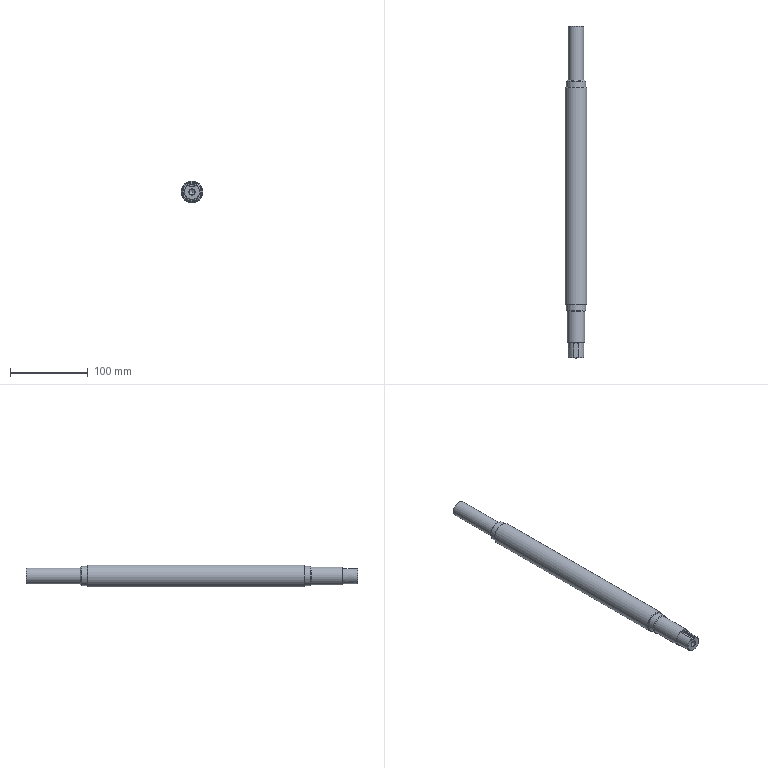Part | NX | features DATUM_CSYS 3, CHAMFER 2, EXTRUDE 2, SKETCH 2, FACE_BLEND 1, HOLE PACKAGE 1, SIMPLE HOLE 1, SWP104 1, SYMBOLIC_THREAD 1 | 1 solid | 25 faces | box 28 x 428 x 28 mm | volume 224992 mm3 | plane 9 | cylinder 8 | cone 8 | commonest cylinder face diameters 20 x2 25 x2 6 x1 7.2 x1 23 x1 28 x1
STEP:
#1=CARTESIAN_POINT('',(0.,428.,9.5));
#2=VERTEX_POINT('',#1);
#3=CARTESIAN_POINT('',(0.,428.,0.));
#4=DIRECTION('',(0.,1.,0.));
#5=DIRECTION('',(0.,0.,1.));
#6=AXIS2_PLACEMENT_3D('',#3,#4,#5);
#7=CIRCLE('',#6,9.5);
#8=EDGE_CURVE('',#2,#2,#7,.T.);
#9=ORIENTED_EDGE('',*,*,#8,.T.);
#10=EDGE_LOOP('',(#9));
#11=FACE_BOUND('',#10,.T.);
#12=CARTESIAN_POINT('',(0.,428.,0.));
#13=DIRECTION('',(0.,1.,0.));
#14=DIRECTION('',(0.,0.,1.));
#15=AXIS2_PLACEMENT_3D('',#12,#13,#14);
#16=PLANE('',#15);
#17=ADVANCED_FACE('',(#11),#16,.T.);
#18=CARTESIAN_POINT('',(0.,427.5,10.));
#19=VERTEX_POINT('',#18);
#20=CARTESIAN_POINT('',(0.,427.5,0.));
#21=DIRECTION('',(0.,1.,0.));
#22=DIRECTION('',(0.,0.,1.));
#23=AXIS2_PLACEMENT_3D('',#20,#21,#22);
#24=CIRCLE('',#23,10.);
#25=EDGE_CURVE('',#19,#19,#24,.F.);
#26=ORIENTED_EDGE('',*,*,#25,.T.);
#27=EDGE_LOOP('',(#26));
#28=FACE_BOUND('',#27,.T.);
#29=CARTESIAN_POINT('',(0.,358.,10.));
#30=VERTEX_POINT('',#29);
#31=CARTESIAN_POINT('',(0.,358.,0.));
#32=DIRECTION('',(0.,1.,0.));
#33=DIRECTION('',(0.,0.,1.));
#34=AXIS2_PLACEMENT_3D('',#31,#32,#33);
#35=CIRCLE('',#34,10.);
#36=EDGE_CURVE('',#30,#30,#35,.T.);
#37=ORIENTED_EDGE('',*,*,#36,.T.);
#38=EDGE_LOOP('',(#37));
#39=FACE_BOUND('',#38,.T.);
#40=CARTESIAN_POINT('',(0.,0.,0.));
#41=DIRECTION('',(0.,1.,0.));
#42=DIRECTION('',(0.,0.,1.));
#43=AXIS2_PLACEMENT_3D('',#40,#41,#42);
#44=CYLINDRICAL_SURFACE('',#43,10.);
#45=ADVANCED_FACE('',(#28,#39),#44,.T.);
#46=CARTESIAN_POINT('',(0.,358.,-11.5));
#47=VERTEX_POINT('',#46);
#48=CARTESIAN_POINT('',(0.,358.,0.));
#49=DIRECTION('',(0.,-1.,0.));
#50=DIRECTION('',(0.,0.,-1.));
#51=AXIS2_PLACEMENT_3D('',#48,#49,#50);
#52=CIRCLE('',#51,11.5);
#53=EDGE_CURVE('',#47,#47,#52,.F.);
#54=ORIENTED_EDGE('',*,*,#53,.T.);
#55=EDGE_LOOP('',(#54));
#56=FACE_BOUND('',#55,.T.);
#57=ORIENTED_EDGE('',*,*,#36,.F.);
#58=EDGE_LOOP('',(#57));
#59=FACE_BOUND('',#58,.T.);
#60=CARTESIAN_POINT('',(-12.5,358.,0.));
#61=DIRECTION('',(0.,-1.,0.));
#62=DIRECTION('',(0.,0.,-1.));
#63=AXIS2_PLACEMENT_3D('',#60,#61,#62);
#64=PLANE('',#63);
#65=ADVANCED_FACE('',(#56,#59),#64,.F.);
#66=CARTESIAN_POINT('',(0.,357.,-12.5));
#67=VERTEX_POINT('',#66);
#68=CARTESIAN_POINT('',(0.,357.,0.));
#69=DIRECTION('',(0.,-1.,0.));
#70=DIRECTION('',(0.,0.,-1.));
#71=AXIS2_PLACEMENT_3D('',#68,#69,#70);
#72=CIRCLE('',#71,12.5);
#73=EDGE_CURVE('',#67,#67,#72,.T.);
#74=ORIENTED_EDGE('',*,*,#73,.T.);
#75=EDGE_LOOP('',(#74));
#76=FACE_BOUND('',#75,.T.);
#77=CARTESIAN_POINT('',(0.,349.,12.5));
#78=VERTEX_POINT('',#77);
#79=CARTESIAN_POINT('',(0.,349.,0.));
#80=DIRECTION('',(0.,1.,0.));
#81=DIRECTION('',(0.,0.,1.));
#82=AXIS2_PLACEMENT_3D('',#79,#80,#81);
#83=CIRCLE('',#82,12.5);
#84=EDGE_CURVE('',#78,#78,#83,.T.);
#85=ORIENTED_EDGE('',*,*,#84,.T.);
#86=EDGE_LOOP('',(#85));
#87=FACE_BOUND('',#86,.T.);
#88=CARTESIAN_POINT('',(0.,0.,0.));
#89=DIRECTION('',(0.,1.,0.));
#90=DIRECTION('',(0.,0.,1.));
#91=AXIS2_PLACEMENT_3D('',#88,#89,#90);
#92=CYLINDRICAL_SURFACE('',#91,12.5);
#93=ADVANCED_FACE('',(#76,#87),#92,.T.);
#94=CARTESIAN_POINT('',(0.,349.,-13.5));
#95=VERTEX_POINT('',#94);
#96=CARTESIAN_POINT('',(0.,349.,0.));
#97=DIRECTION('',(0.,-1.,0.));
#98=DIRECTION('',(0.,0.,-1.));
#99=AXIS2_PLACEMENT_3D('',#96,#97,#98);
#100=CIRCLE('',#99,13.5);
#101=EDGE_CURVE('',#95,#95,#100,.F.);
#102=ORIENTED_EDGE('',*,*,#101,.T.);
#103=EDGE_LOOP('',(#102));
#104=FACE_BOUND('',#103,.T.);
#105=ORIENTED_EDGE('',*,*,#84,.F.);
#106=EDGE_LOOP('',(#105));
#107=FACE_BOUND('',#106,.T.);
#108=CARTESIAN_POINT('',(-14.,349.,0.));
#109=DIRECTION('',(0.,-1.,0.));
#110=DIRECTION('',(0.,0.,-1.));
#111=AXIS2_PLACEMENT_3D('',#108,#109,#110);
#112=PLANE('',#111);
#113=ADVANCED_FACE('',(#104,#107),#112,.F.);
#114=CARTESIAN_POINT('',(0.,348.5,-14.));
#115=VERTEX_POINT('',#114);
#116=CARTESIAN_POINT('',(0.,348.5,0.));
#117=DIRECTION('',(0.,-1.,0.));
#118=DIRECTION('',(0.,0.,-1.));
#119=AXIS2_PLACEMENT_3D('',#116,#117,#118);
#120=CIRCLE('',#119,14.);
#121=EDGE_CURVE('',#115,#115,#120,.T.);
#122=ORIENTED_EDGE('',*,*,#121,.T.);
#123=EDGE_LOOP('',(#122));
#124=FACE_BOUND('',#123,.T.);
#125=CARTESIAN_POINT('',(0.,69.5,14.));
#126=VERTEX_POINT('',#125);
#127=CARTESIAN_POINT('',(0.,69.5,0.));
#128=DIRECTION('',(0.,1.,0.));
#129=DIRECTION('',(0.,0.,1.));
#130=AXIS2_PLACEMENT_3D('',#127,#128,#129);
#131=CIRCLE('',#130,14.);
#132=EDGE_CURVE('',#126,#126,#131,.T.);
#133=ORIENTED_EDGE('',*,*,#132,.T.);
#134=EDGE_LOOP('',(#133));
#135=FACE_BOUND('',#134,.T.);
#136=CARTESIAN_POINT('',(0.,0.,0.));
#137=DIRECTION('',(0.,1.,0.));
#138=DIRECTION('',(0.,0.,1.));
#139=AXIS2_PLACEMENT_3D('',#136,#137,#138);
#140=CYLINDRICAL_SURFACE('',#139,14.);
#141=ADVANCED_FACE('',(#124,#135),#140,.T.);
#142=CARTESIAN_POINT('',(0.,69.,13.5));
#143=VERTEX_POINT('',#142);
#144=CARTESIAN_POINT('',(0.,69.,0.));
#145=DIRECTION('',(0.,1.,0.));
#146=DIRECTION('',(0.,0.,1.));
#147=AXIS2_PLACEMENT_3D('',#144,#145,#146);
#148=CIRCLE('',#147,13.5);
#149=EDGE_CURVE('',#143,#143,#148,.F.);
#150=ORIENTED_EDGE('',*,*,#149,.T.);
#151=EDGE_LOOP('',(#150));
#152=FACE_BOUND('',#151,.T.);
#153=CARTESIAN_POINT('',(0.,69.,12.5));
#154=VERTEX_POINT('',#153);
#155=CARTESIAN_POINT('',(0.,69.,0.));
#156=DIRECTION('',(0.,1.,0.));
#157=DIRECTION('',(0.,0.,1.));
#158=AXIS2_PLACEMENT_3D('',#155,#156,#157);
#159=CIRCLE('',#158,12.5);
#160=EDGE_CURVE('',#154,#154,#159,.T.);
#161=ORIENTED_EDGE('',*,*,#160,.T.);
#162=EDGE_LOOP('',(#161));
#163=FACE_BOUND('',#162,.T.);
#164=CARTESIAN_POINT('',(-12.5,69.,0.));
#165=DIRECTION('',(0.,1.,0.));
#166=DIRECTION('',(0.,0.,1.));
#167=AXIS2_PLACEMENT_3D('',#164,#165,#166);
#168=PLANE('',#167);
#169=ADVANCED_FACE('',(#152,#163),#168,.F.);
#170=CARTESIAN_POINT('',(0.,61.,12.5));
#171=VERTEX_POINT('',#170);
#172=CARTESIAN_POINT('',(0.,61.,0.));
#173=DIRECTION('',(0.,1.,0.));
#174=DIRECTION('',(0.,0.,1.));
#175=AXIS2_PLACEMENT_3D('',#172,#173,#174);
#176=CIRCLE('',#175,12.5);
#177=EDGE_CURVE('',#171,#171,#176,.T.);
#178=ORIENTED_EDGE('',*,*,#177,.T.);
#179=EDGE_LOOP('',(#178));
#180=FACE_BOUND('',#179,.T.);
#181=ORIENTED_EDGE('',*,*,#160,.F.);
#182=EDGE_LOOP('',(#181));
#183=FACE_BOUND('',#182,.T.);
#184=CARTESIAN_POINT('',(0.,0.,0.));
#185=DIRECTION('',(0.,1.,0.));
#186=DIRECTION('',(0.,0.,1.));
#187=AXIS2_PLACEMENT_3D('',#184,#185,#186);
#188=CYLINDRICAL_SURFACE('',#187,12.5);
#189=ADVANCED_FACE('',(#180,#183),#188,.T.);
#190=ORIENTED_EDGE('',*,*,#25,.F.);
#191=EDGE_LOOP('',(#190));
#192=FACE_BOUND('',#191,.T.);
#193=ORIENTED_EDGE('',*,*,#8,.F.);
#194=EDGE_LOOP('',(#193));
#195=FACE_BOUND('',#194,.T.);
#196=CARTESIAN_POINT('',(0.,428.,0.));
#197=DIRECTION('',(0.,-1.,0.));
#198=DIRECTION('',(0.,0.,-1.));
#199=AXIS2_PLACEMENT_3D('',#196,#197,#198);
#200=CONICAL_SURFACE('',#199,9.5,0.7854);
#201=ADVANCED_FACE('',(#192,#195),#200,.T.);
#202=ORIENTED_EDGE('',*,*,#121,.F.);
#203=EDGE_LOOP('',(#202));
#204=FACE_BOUND('',#203,.T.);
#205=ORIENTED_EDGE('',*,*,#101,.F.);
#206=EDGE_LOOP('',(#205));
#207=FACE_BOUND('',#206,.T.);
#208=CARTESIAN_POINT('',(0.,349.,0.));
#209=DIRECTION('',(0.,-1.,0.));
#210=DIRECTION('',(0.,0.,-1.));
#211=AXIS2_PLACEMENT_3D('',#208,#209,#210);
#212=CONICAL_SURFACE('',#211,13.5,0.7854);
#213=ADVANCED_FACE('',(#204,#207),#212,.T.);
#214=ORIENTED_EDGE('',*,*,#149,.F.);
#215=EDGE_LOOP('',(#214));
#216=FACE_BOUND('',#215,.T.);
#217=ORIENTED_EDGE('',*,*,#132,.F.);
#218=EDGE_LOOP('',(#217));
#219=FACE_BOUND('',#218,.T.);
#220=CARTESIAN_POINT('',(0.,69.5,0.));
#221=DIRECTION('',(0.,1.,0.));
#222=DIRECTION('',(0.,0.,1.));
#223=AXIS2_PLACEMENT_3D('',#220,#221,#222);
#224=CONICAL_SURFACE('',#223,14.,0.7854);
#225=ADVANCED_FACE('',(#216,#219),#224,.T.);
#226=CARTESIAN_POINT('',(0.,60.,11.5));
#227=VERTEX_POINT('',#226);
#228=CARTESIAN_POINT('',(0.,60.,0.));
#229=DIRECTION('',(0.,1.,0.));
#230=DIRECTION('',(0.,0.,1.));
#231=AXIS2_PLACEMENT_3D('',#228,#229,#230);
#232=CIRCLE('',#231,11.5);
#233=EDGE_CURVE('',#227,#227,#232,.F.);
#234=ORIENTED_EDGE('',*,*,#233,.F.);
#235=EDGE_LOOP('',(#234));
#236=FACE_BOUND('',#235,.T.);
#237=ORIENTED_EDGE('',*,*,#177,.F.);
#238=EDGE_LOOP('',(#237));
#239=FACE_BOUND('',#238,.T.);
#240=CARTESIAN_POINT('',(0.,61.,0.));
#241=DIRECTION('',(0.,1.,0.));
#242=DIRECTION('',(0.,0.,1.));
#243=AXIS2_PLACEMENT_3D('',#240,#241,#242);
#244=CONICAL_SURFACE('',#243,12.5,0.7854);
#245=ADVANCED_FACE('',(#236,#239),#244,.T.);
#246=ORIENTED_EDGE('',*,*,#73,.F.);
#247=EDGE_LOOP('',(#246));
#248=FACE_BOUND('',#247,.T.);
#249=ORIENTED_EDGE('',*,*,#53,.F.);
#250=EDGE_LOOP('',(#249));
#251=FACE_BOUND('',#250,.T.);
#252=CARTESIAN_POINT('',(0.,358.,0.));
#253=DIRECTION('',(0.,-1.,0.));
#254=DIRECTION('',(0.,0.,-1.));
#255=AXIS2_PLACEMENT_3D('',#252,#253,#254);
#256=CONICAL_SURFACE('',#255,11.5,0.7854);
#257=ADVANCED_FACE('',(#248,#251),#256,.T.);
#258=CARTESIAN_POINT('',(0.,20.,-11.5));
#259=VERTEX_POINT('',#258);
#260=CARTESIAN_POINT('',(0.,20.,0.));
#261=DIRECTION('',(0.,-1.,0.));
#262=DIRECTION('',(0.,0.,-1.));
#263=AXIS2_PLACEMENT_3D('',#260,#261,#262);
#264=CIRCLE('',#263,11.5);
#265=EDGE_CURVE('',#259,#259,#264,.T.);
#266=ORIENTED_EDGE('',*,*,#265,.T.);
#267=EDGE_LOOP('',(#266));
#268=FACE_BOUND('',#267,.T.);
#269=CARTESIAN_POINT('',(0.,20.,10.));
#270=VERTEX_POINT('',#269);
#271=CARTESIAN_POINT('',(0.,20.,0.));
#272=DIRECTION('',(0.,-1.,0.));
#273=DIRECTION('',(0.,0.,-1.));
#274=AXIS2_PLACEMENT_3D('',#271,#272,#273);
#275=CIRCLE('',#274,10.);
#276=EDGE_CURVE('',#270,#270,#275,.T.);
#277=ORIENTED_EDGE('',*,*,#276,.F.);
#278=EDGE_LOOP('',(#277));
#279=FACE_BOUND('',#278,.T.);
#280=CARTESIAN_POINT('',(0.,20.,0.));
#281=DIRECTION('',(0.,-1.,0.));
#282=DIRECTION('',(0.,0.,-1.));
#283=AXIS2_PLACEMENT_3D('',#280,#281,#282);
#284=PLANE('',#283);
#285=ADVANCED_FACE('',(#268,#279),#284,.T.);
#286=ORIENTED_EDGE('',*,*,#265,.F.);
#287=EDGE_LOOP('',(#286));
#288=FACE_BOUND('',#287,.T.);
#289=ORIENTED_EDGE('',*,*,#233,.T.);
#290=EDGE_LOOP('',(#289));
#291=FACE_BOUND('',#290,.T.);
#292=CARTESIAN_POINT('',(0.,20.,0.));
#293=DIRECTION('',(0.,1.,0.));
#294=DIRECTION('',(0.,0.,1.));
#295=AXIS2_PLACEMENT_3D('',#292,#293,#294);
#296=CYLINDRICAL_SURFACE('',#295,11.5);
#297=ADVANCED_FACE('',(#288,#291),#296,.T.);
#298=CARTESIAN_POINT('',(0.,15.,3.6));
#299=VERTEX_POINT('',#298);
#300=CARTESIAN_POINT('',(0.,15.,0.));
#301=DIRECTION('',(0.,1.,0.));
#302=DIRECTION('',(0.,0.,1.));
#303=AXIS2_PLACEMENT_3D('',#300,#301,#302);
#304=CIRCLE('',#303,3.6);
#305=EDGE_CURVE('',#299,#299,#304,.F.);
#306=ORIENTED_EDGE('',*,*,#305,.T.);
#307=EDGE_LOOP('',(#306));
#308=FACE_BOUND('',#307,.T.);
#309=CARTESIAN_POINT('',(0.,17.163,0.));
#310=VERTEX_POINT('',#309);
#311=VERTEX_LOOP('',#310);
#312=FACE_BOUND('',#311,.T.);
#313=CARTESIAN_POINT('',(0.,15.,0.));
#314=DIRECTION('',(0.,-1.,0.));
#315=DIRECTION('',(0.,0.,-1.));
#316=AXIS2_PLACEMENT_3D('',#313,#314,#315);
#317=CONICAL_SURFACE('',#316,3.6,1.03);
#318=ADVANCED_FACE('',(#308,#312),#317,.F.);
#319=CARTESIAN_POINT('',(0.,0.4,3.6));
#320=VERTEX_POINT('',#319);
#321=CARTESIAN_POINT('',(0.,0.4,0.));
#322=DIRECTION('',(0.,1.,0.));
#323=DIRECTION('',(0.,0.,1.));
#324=AXIS2_PLACEMENT_3D('',#321,#322,#323);
#325=CIRCLE('',#324,3.6);
#326=EDGE_CURVE('',#320,#320,#325,.F.);
#327=ORIENTED_EDGE('',*,*,#326,.T.);
#328=EDGE_LOOP('',(#327));
#329=FACE_BOUND('',#328,.T.);
#330=ORIENTED_EDGE('',*,*,#305,.F.);
#331=EDGE_LOOP('',(#330));
#332=FACE_BOUND('',#331,.T.);
#333=CARTESIAN_POINT('',(0.,0.,0.));
#334=DIRECTION('',(0.,1.,0.));
#335=DIRECTION('',(0.,0.,1.));
#336=AXIS2_PLACEMENT_3D('',#333,#334,#335);
#337=CYLINDRICAL_SURFACE('',#336,3.6);
#338=ADVANCED_FACE('',(#329,#332),#337,.F.);
#339=ORIENTED_EDGE('',*,*,#326,.F.);
#340=EDGE_LOOP('',(#339));
#341=FACE_BOUND('',#340,.T.);
#342=CARTESIAN_POINT('',(0.,0.,4.));
#343=VERTEX_POINT('',#342);
#344=CARTESIAN_POINT('',(0.,0.,0.));
#345=DIRECTION('',(0.,1.,0.));
#346=DIRECTION('',(0.,0.,1.));
#347=AXIS2_PLACEMENT_3D('',#344,#345,#346);
#348=CIRCLE('',#347,4.);
#349=EDGE_CURVE('',#343,#343,#348,.T.);
#350=ORIENTED_EDGE('',*,*,#349,.F.);
#351=EDGE_LOOP('',(#350));
#352=FACE_BOUND('',#351,.T.);
#353=CARTESIAN_POINT('',(0.,0.,0.));
#354=DIRECTION('',(0.,-1.,0.));
#355=DIRECTION('',(0.,0.,-1.));
#356=AXIS2_PLACEMENT_3D('',#353,#354,#355);
#357=CONICAL_SURFACE('',#356,4.,0.7854);
#358=ADVANCED_FACE('',(#341,#352),#357,.F.);
#359=ORIENTED_EDGE('',*,*,#349,.T.);
#360=EDGE_LOOP('',(#359));
#361=FACE_BOUND('',#360,.T.);
#362=CARTESIAN_POINT('',(-3.,0.,9.014));
#363=VERTEX_POINT('',#362);
#364=CARTESIAN_POINT('',(-3.,0.,6.5));
#365=VERTEX_POINT('',#364);
#366=CARTESIAN_POINT('',(-3.,0.,21.5));
#367=DIRECTION('',(0.,0.,-1.));
#368=VECTOR('',#367,1000.);
#369=LINE('',#366,#368);
#370=EDGE_CURVE('',#363,#365,#369,.T.);
#371=ORIENTED_EDGE('',*,*,#370,.F.);
#372=CARTESIAN_POINT('',(3.,0.,9.014));
#373=VERTEX_POINT('',#372);
#374=CARTESIAN_POINT('',(0.,0.,0.));
#375=DIRECTION('',(0.,1.,0.));
#376=DIRECTION('',(0.,0.,1.));
#377=AXIS2_PLACEMENT_3D('',#374,#375,#376);
#378=CIRCLE('',#377,9.5);
#379=EDGE_CURVE('',#363,#373,#378,.F.);
#380=ORIENTED_EDGE('',*,*,#379,.T.);
#381=CARTESIAN_POINT('',(3.,0.,6.5));
#382=VERTEX_POINT('',#381);
#383=CARTESIAN_POINT('',(3.,0.,6.5));
#384=DIRECTION('',(0.,0.,1.));
#385=VECTOR('',#384,1000.);
#386=LINE('',#383,#385);
#387=EDGE_CURVE('',#382,#373,#386,.T.);
#388=ORIENTED_EDGE('',*,*,#387,.F.);
#389=CARTESIAN_POINT('',(-3.,0.,6.5));
#390=DIRECTION('',(1.,0.,0.));
#391=VECTOR('',#390,1000.);
#392=LINE('',#389,#391);
#393=EDGE_CURVE('',#365,#382,#392,.T.);
#394=ORIENTED_EDGE('',*,*,#393,.F.);
#395=EDGE_LOOP('',(#371,#380,#388,#394));
#396=FACE_BOUND('',#395,.T.);
#397=CARTESIAN_POINT('',(0.,0.,0.));
#398=DIRECTION('',(0.,1.,0.));
#399=DIRECTION('',(0.,0.,1.));
#400=AXIS2_PLACEMENT_3D('',#397,#398,#399);
#401=PLANE('',#400);
#402=ADVANCED_FACE('',(#361,#396),#401,.F.);
#403=CARTESIAN_POINT('',(3.,17.,6.5));
#404=VERTEX_POINT('',#403);
#405=CARTESIAN_POINT('',(3.,20.,6.5));
#406=DIRECTION('',(0.,-1.,0.));
#407=VECTOR('',#406,1000.);
#408=LINE('',#405,#407);
#409=EDGE_CURVE('',#382,#404,#408,.F.);
#410=ORIENTED_EDGE('',*,*,#409,.T.);
#411=CARTESIAN_POINT('',(-3.,17.,6.5));
#412=VERTEX_POINT('',#411);
#413=CARTESIAN_POINT('',(0.,17.,6.5));
#414=DIRECTION('',(0.,0.,-1.));
#415=DIRECTION('',(-1.,0.,0.));
#416=AXIS2_PLACEMENT_3D('',#413,#414,#415);
#417=CIRCLE('',#416,3.);
#418=EDGE_CURVE('',#404,#412,#417,.F.);
#419=ORIENTED_EDGE('',*,*,#418,.T.);
#420=CARTESIAN_POINT('',(-3.,20.,6.5));
#421=DIRECTION('',(0.,-1.,0.));
#422=VECTOR('',#421,1000.);
#423=LINE('',#420,#422);
#424=EDGE_CURVE('',#365,#412,#423,.F.);
#425=ORIENTED_EDGE('',*,*,#424,.F.);
#426=ORIENTED_EDGE('',*,*,#393,.T.);
#427=EDGE_LOOP('',(#410,#419,#425,#426));
#428=FACE_BOUND('',#427,.T.);
#429=CARTESIAN_POINT('',(-3.,20.,6.5));
#430=DIRECTION('',(0.,0.,-1.));
#431=DIRECTION('',(-1.,0.,0.));
#432=AXIS2_PLACEMENT_3D('',#429,#430,#431);
#433=PLANE('',#432);
#434=ADVANCED_FACE('',(#428),#433,.F.);
#435=CARTESIAN_POINT('',(-3.,0.5,9.539));
#436=VERTEX_POINT('',#435);
#437=CARTESIAN_POINT('',(-3.,17.,9.539));
#438=VERTEX_POINT('',#437);
#439=CARTESIAN_POINT('',(-3.,0.,9.539));
#440=DIRECTION('',(0.,1.,0.));
#441=VECTOR('',#440,1000.);
#442=LINE('',#439,#441);
#443=EDGE_CURVE('',#436,#438,#442,.T.);
#444=ORIENTED_EDGE('',*,*,#443,.F.);
#445=CARTESIAN_POINT('',(-3.,0.5,9.539));
#446=CARTESIAN_POINT('',(-3.,0.3331,9.364));
#447=CARTESIAN_POINT('',(-3.,0.1664,9.189));
#448=CARTESIAN_POINT('',(-3.,0.,9.014));
#449=B_SPLINE_CURVE_WITH_KNOTS('',3,(#445,#446,#447,#448),.UNSPECIFIED.,.F.,.F.,(4,4),(0.,0.0007254),.UNSPECIFIED.);
#450=EDGE_CURVE('',#436,#363,#449,.T.);
#451=ORIENTED_EDGE('',*,*,#450,.T.);
#452=ORIENTED_EDGE('',*,*,#370,.T.);
#453=ORIENTED_EDGE('',*,*,#424,.T.);
#454=CARTESIAN_POINT('',(-3.,17.,21.5));
#455=DIRECTION('',(0.,0.,-1.));
#456=VECTOR('',#455,1000.);
#457=LINE('',#454,#456);
#458=EDGE_CURVE('',#412,#438,#457,.F.);
#459=ORIENTED_EDGE('',*,*,#458,.T.);
#460=EDGE_LOOP('',(#444,#451,#452,#453,#459));
#461=FACE_BOUND('',#460,.T.);
#462=CARTESIAN_POINT('',(-3.,20.,21.5));
#463=DIRECTION('',(-1.,0.,0.));
#464=DIRECTION('',(0.,0.,1.));
#465=AXIS2_PLACEMENT_3D('',#462,#463,#464);
#466=PLANE('',#465);
#467=ADVANCED_FACE('',(#461),#466,.F.);
#468=CARTESIAN_POINT('',(3.,0.5,9.539));
#469=VERTEX_POINT('',#468);
#470=CARTESIAN_POINT('',(3.,0.,9.014));
#471=CARTESIAN_POINT('',(3.,0.1664,9.189));
#472=CARTESIAN_POINT('',(3.,0.3331,9.364));
#473=CARTESIAN_POINT('',(3.,0.5,9.539));
#474=B_SPLINE_CURVE_WITH_KNOTS('',3,(#470,#471,#472,#473),.UNSPECIFIED.,.F.,.F.,(4,4),(0.,0.0007254),.UNSPECIFIED.);
#475=EDGE_CURVE('',#373,#469,#474,.T.);
#476=ORIENTED_EDGE('',*,*,#475,.F.);
#477=ORIENTED_EDGE('',*,*,#379,.F.);
#478=ORIENTED_EDGE('',*,*,#450,.F.);
#479=CARTESIAN_POINT('',(0.,0.5,0.));
#480=DIRECTION('',(0.,1.,0.));
#481=DIRECTION('',(0.,0.,1.));
#482=AXIS2_PLACEMENT_3D('',#479,#480,#481);
#483=CIRCLE('',#482,10.);
#484=EDGE_CURVE('',#469,#436,#483,.T.);
#485=ORIENTED_EDGE('',*,*,#484,.F.);
#486=EDGE_LOOP('',(#476,#477,#478,#485));
#487=FACE_BOUND('',#486,.T.);
#488=CARTESIAN_POINT('',(0.,0.5,0.));
#489=DIRECTION('',(0.,1.,0.));
#490=DIRECTION('',(0.,0.,1.));
#491=AXIS2_PLACEMENT_3D('',#488,#489,#490);
#492=CONICAL_SURFACE('',#491,10.,0.7854);
#493=ADVANCED_FACE('',(#487),#492,.T.);
#494=ORIENTED_EDGE('',*,*,#387,.T.);
#495=ORIENTED_EDGE('',*,*,#475,.T.);
#496=CARTESIAN_POINT('',(3.,17.,9.539));
#497=VERTEX_POINT('',#496);
#498=CARTESIAN_POINT('',(3.,0.,9.539));
#499=DIRECTION('',(0.,1.,0.));
#500=VECTOR('',#499,1000.);
#501=LINE('',#498,#500);
#502=EDGE_CURVE('',#497,#469,#501,.F.);
#503=ORIENTED_EDGE('',*,*,#502,.F.);
#504=CARTESIAN_POINT('',(3.,17.,6.5));
#505=DIRECTION('',(0.,0.,-1.));
#506=VECTOR('',#505,1000.);
#507=LINE('',#504,#506);
#508=EDGE_CURVE('',#497,#404,#507,.T.);
#509=ORIENTED_EDGE('',*,*,#508,.T.);
#510=ORIENTED_EDGE('',*,*,#409,.F.);
#511=EDGE_LOOP('',(#494,#495,#503,#509,#510));
#512=FACE_BOUND('',#511,.T.);
#513=CARTESIAN_POINT('',(3.,20.,6.5));
#514=DIRECTION('',(1.,0.,0.));
#515=DIRECTION('',(0.,0.,-1.));
#516=AXIS2_PLACEMENT_3D('',#513,#514,#515);
#517=PLANE('',#516);
#518=ADVANCED_FACE('',(#512),#517,.F.);
#519=ORIENTED_EDGE('',*,*,#458,.F.);
#520=ORIENTED_EDGE('',*,*,#418,.F.);
#521=ORIENTED_EDGE('',*,*,#508,.F.);
#522=CARTESIAN_POINT('',(0.,20.,10.));
#523=CARTESIAN_POINT('',(0.7973,20.,10.));
#524=CARTESIAN_POINT('',(2.343,19.345,9.775));
#525=CARTESIAN_POINT('',(3.,17.797,9.539));
#526=CARTESIAN_POINT('',(3.,17.,9.539));
#527=B_SPLINE_CURVE_WITH_KNOTS('',3,(#522,#523,#524,#525,#526),.UNSPECIFIED.,.F.,.F.,(4,1,4),(0.004714,0.007071,0.009428),.UNSPECIFIED.);
#528=EDGE_CURVE('',#497,#270,#527,.F.);
#529=ORIENTED_EDGE('',*,*,#528,.T.);
#530=CARTESIAN_POINT('',(-3.,17.,9.539));
#531=CARTESIAN_POINT('',(-3.,17.797,9.539));
#532=CARTESIAN_POINT('',(-2.345,19.343,9.775));
#533=CARTESIAN_POINT('',(-0.7973,20.,10.));
#534=CARTESIAN_POINT('',(0.,20.,10.));
#535=B_SPLINE_CURVE_WITH_KNOTS('',3,(#530,#531,#532,#533,#534),.UNSPECIFIED.,.F.,.F.,(4,1,4),(0.,0.002357,0.004714),.UNSPECIFIED.);
#536=EDGE_CURVE('',#270,#438,#535,.F.);
#537=ORIENTED_EDGE('',*,*,#536,.T.);
#538=EDGE_LOOP('',(#519,#520,#521,#529,#537));
#539=FACE_BOUND('',#538,.T.);
#540=CARTESIAN_POINT('',(0.,17.,9.539));
#541=DIRECTION('',(0.,0.,-1.));
#542=DIRECTION('',(0.,1.,0.));
#543=AXIS2_PLACEMENT_3D('',#540,#541,#542);
#544=CYLINDRICAL_SURFACE('',#543,3.);
#545=ADVANCED_FACE('',(#539),#544,.F.);
#546=ORIENTED_EDGE('',*,*,#536,.F.);
#547=ORIENTED_EDGE('',*,*,#276,.T.);
#548=ORIENTED_EDGE('',*,*,#528,.F.);
#549=ORIENTED_EDGE('',*,*,#502,.T.);
#550=ORIENTED_EDGE('',*,*,#484,.T.);
#551=ORIENTED_EDGE('',*,*,#443,.T.);
#552=EDGE_LOOP('',(#546,#547,#548,#549,#550,#551));
#553=FACE_BOUND('',#552,.T.);
#554=CARTESIAN_POINT('',(0.,0.,0.));
#555=DIRECTION('',(0.,1.,0.));
#556=DIRECTION('',(0.,0.,1.));
#557=AXIS2_PLACEMENT_3D('',#554,#555,#556);
#558=CYLINDRICAL_SURFACE('',#557,10.);
#559=ADVANCED_FACE('',(#553),#558,.T.);
#560=CLOSED_SHELL('',(#17,#45,#65,#93,#113,#141,#169,#189,#201,#213,#225,#245,#257,#285,#297,#318,#338,#358,#402,#434,#467,#493,#518,#545,#559));
#561=MANIFOLD_SOLID_BREP('',#560);
#562=(LENGTH_UNIT()NAMED_UNIT(*)SI_UNIT(.MILLI.,.METRE.));
#563=UNCERTAINTY_MEASURE_WITH_UNIT(LENGTH_MEASURE(0.0508),#562,'','');
#564=(NAMED_UNIT(*)PLANE_ANGLE_UNIT()SI_UNIT($,.RADIAN.));
#565=(NAMED_UNIT(*)SI_UNIT($,.STERADIAN.)SOLID_ANGLE_UNIT());
#566=(GEOMETRIC_REPRESENTATION_CONTEXT(3)GLOBAL_UNCERTAINTY_ASSIGNED_CONTEXT((#563))GLOBAL_UNIT_ASSIGNED_CONTEXT((#562,#564,#565))REPRESENTATION_CONTEXT('',''));
#567=ADVANCED_BREP_SHAPE_REPRESENTATION('',(#561),#566);